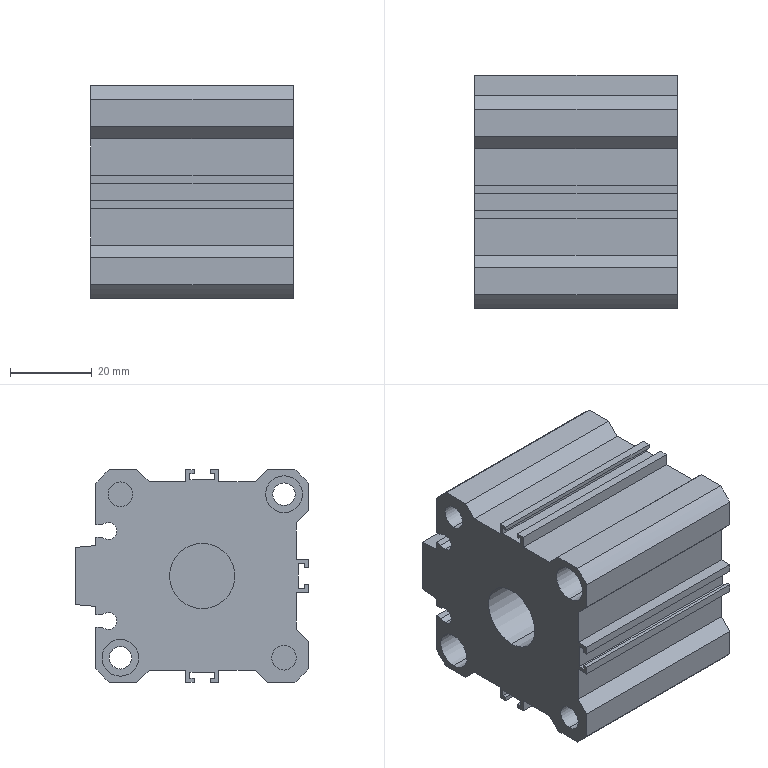Part | STEP file | 1105WWT1_1 | 1 solid | 114 faces | box 49.5 x 57 x 52 mm | volume 94485 mm3 | plane 72 | cylinder 34 | cone 8 | commonest cylinder face diameters 9 x8 4.15 x6 5.5 x4 6 x4 8.566 x4 69 x4